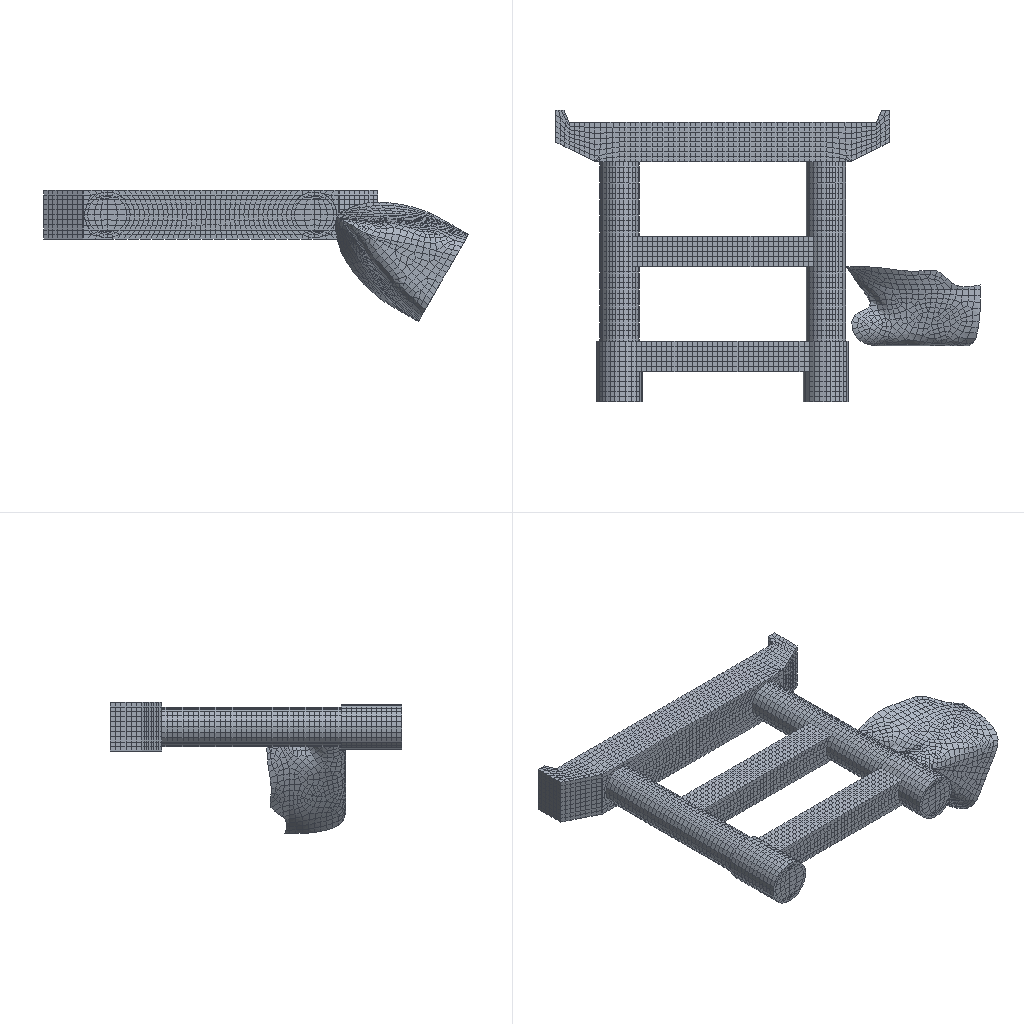Simulation study | abaqus
Set-up summary:
category,name,step,type,value,unit,region
solver,abaqus
solver,version,,,Abaqus/Explicit 2024
units,not stated in the deck,,not stated
analysis,deck,,transient,transient
load_step,Step-1,Step-1,transient,nlgeom=True
contact,interactions,,,general=1 pairs=0 ties=0
load_step,requested,,,1
mesh,nodes,,,29370
mesh,elements,,,26908
element_type,S3,,shell,56
element_type,S4R,,shell,1150
element_type,T3D2,,truss,11894
element_type,C3D8R,,solid,13808
load,load commands in deck,,count,1
bc,support commands in deck,,count,2
material,C40,,in results
material,HRE335,,in results
material,SHIP,,in results
check,setup vs results,,match,"per instance, exact: element labels, types and connectivity; labels of the nodes the elements use; coordinates of those nodes at SINGLE_PRECISION in 1 of 3 instance(s)"
Abaqus input file, long lists of numbers shortened:
*Heading
** Job name: Job-2 Model name: Model-1-Copy
** Generated by: Abaqus/CAE 2024
*Preprint, echo=NO, model=NO, history=NO, contact=NO
**
** PARTS
**
*Part, name=Bow
*Node
      1,   37800.219,        9242.,           0.
      2,       37800.,        9242.,           0.
** (1225 more lines like these left out)
*Element, type=S3
1,  47,  46,   4
2,  44,  49, 273
** (54 more lines like these left out)
*Element, type=S4R
  5,  19,  20, 352, 358
  6, 349,  64,  65, 358
** (1148 more lines like these left out)
*Nset, nset=BOW
 4,
*Nset, nset=Set-2, generate
    1,  1227,     1
*Elset, elset=Set-2, generate
    1,  1206,     1
*Nset, nset=Set-3, generate
    1,  1227,     1
** Section: Section-3
*Shell Section, elset=Set-2, material=Ship
50., 5
*End Part
**
*Part, name=Concrete
*Node
      1,       27500.,       -1500.,      -32750.
      2,       27500.,       -4000.,      -32750.
** (17351 more lines like these left out)
*Element, type=C3D8R
  1,     1,   285,  3364,   298,   329,  3544, 11654,  3384
  2,   285,   286,  3365,  3364,  3544,  3545, 11655, 11654
** (13806 more lines like these left out)
*Nset, nset=Set-1, generate
     1,  17353,      1
*Elset, elset=Set-1, generate
     1,  13808,      1
** Section: C40
*Solid Section, elset=Set-1, material=C40
,
*End Part
**
*Part, name=ganfjinlong
*Node
      1,      127050.,      -37500.,        4000.
      2,      130050.,      -37500.,        4000.
** (10788 more lines like these left out)
*Element, type=T3D2
1,    1, 1237
2, 1237, 1238
** (11892 more lines like these left out)
*Nset, nset=Set-1, generate
     1,  10790,      1
*Elset, elset=Set-1, generate
     1,  11894,      1
*Nset, nset=Set-2
   793,   794,   795,   796,   797,   798,   799,   800,   801,   802,   803,   804,   805,   806,   807,   808
   809,   810,   811,   812,   813,   814,   815,   816,   817,   818,   819,   820,   821,   822,   823,   824
** (225 more lines like these left out)
*Elset, elset=Set-2, generate
  7869,  11894,      1
** Section: HRB335
*Solid Section, elset=Set-1, material=HRE335
50.35,
*End Part
**
**
** ASSEMBLY
**
*Assembly, name=Assembly
**
*Instance, name=Concrete-1, part=Concrete
     116550.,           0.,           0.
     116550.,           0.,           0., 116549.,           0.,           0., 90.
*End Instance
**
*Instance, name=ganfjinlong-1, part=ganfjinlong
*End Instance
**
*Instance, name=Bow-1, part=Bow
215030.036,      -33500., -25289.
215030.036,      -33500., -25289., 215030.036, -33499., -25289., 210.
*End Instance
**
*Node
      1,   182294.281,      -24258.,       -6389.
*Nset, nset=Set-6, instance=Concrete-1
   235,   237,   238,   240,   241,   242,   243,   244,   245,   246,   247,   248,   249,   250,   251,   252
   253,   254,   255,   257,   260,   261,   262,   263,   265,   267,   268,   269,   270,   271,   273,   274
** (10 more lines like these left out)
*Elset, elset=Set-6, instance=Concrete-1
 10779, 10791, 10803, 10815, 10827, 10839, 10851, 10863, 10875, 10887, 10899, 10911, 10923, 10935, 10947, 10959
 10971, 10983, 11006, 11018, 11030, 11031, 11043, 11055, 11067, 11079, 11091, 11103, 11115, 11127, 11172, 11173
** (9 more lines like these left out)
*Nset, nset=Set-7, instance=Concrete-1
   37,   39,   40,   46,   54,   55,   56,   71,   74,   75,   78,   79,   81,   83,   85,   99
  100,  137,  141,  145,  169,  170,  172,  828,  829,  832,  866,  867, 1014, 1015, 1016, 1278
** (8 more lines like these left out)
*Elset, elset=Set-7, instance=Concrete-1
 4435, 4442, 4449, 4456, 4463, 4470, 4477, 4484, 4491, 4498, 4505, 4512, 4519, 4526, 4533, 4540
 4547, 4554, 4561, 4568, 4575, 4582, 4589, 4596, 4603, 4610, 4617, 4624, 4631, 4638, 4645, 4652
** (7 more lines like these left out)
*Nset, nset=Set-11, instance=Bow-1, generate
    1,  1227,     1
*Elset, elset=Set-11, instance=Bow-1, generate
    1,  1206,     1
*Nset, nset=m_Set-3, instance=ganfjinlong-1, generate
     1,  10790,      1
*Elset, elset=m_Set-3, instance=ganfjinlong-1, generate
     1,  11894,      1
*Nset, nset=m_Set-10, instance=ganfjinlong-1, generate
     1,  10790,      1
*Elset, elset=m_Set-10, instance=ganfjinlong-1, generate
     1,  11894,      1
*Nset, nset=s_Set-3, instance=Concrete-1, generate
     1,  17353,      1
*Elset, elset=s_Set-3, instance=Concrete-1, generate
     1,  13808,      1
*Nset, nset=s_Set-10, instance=Concrete-1, generate
     1,  17353,      1
*Elset, elset=s_Set-10, instance=Concrete-1, generate
     1,  13808,      1
*Nset, nset=_PickedSet378, internal
 1,
*Nset, nset=_PickedSet379, internal, instance=Bow-1, generate
    1,  1227,     1
*Elset, elset=_PickedSet379, internal, instance=Bow-1, generate
    1,  1206,     1
*Nset, nset=_PickedSet380, internal
 1,
*Elset, elset=_m_Surf-1_SNEG, internal, instance=Bow-1, generate
    1,  1206,     1
*Surface, type=ELEMENT, name=m_Surf-1
_m_Surf-1_SNEG, SNEG
*Elset, elset=_m_Surf-3_SNEG, internal, instance=Bow-1, generate
    1,  1206,     1
*Surface, type=ELEMENT, name=m_Surf-3
_m_Surf-3_SNEG, SNEG
*Elset, elset=_s_Surf-1_S3, internal, instance=Concrete-1
  7175,  7176,  7177,  7184,  7185,  7186,  7193,  7194,  7195,  7202,  7203,  7204,  7211,  7212,  7213,  7220
  7221,  7222,  7229,  7230,  7231,  7238,  7239,  7240,  7247,  7248,  7249,  7256,  7257,  7258,  7265,  7266
** (4 more lines like these left out)
*Elset, elset=_s_Surf-1_S6, internal, instance=Concrete-1
 7301, 7304, 7307, 7310, 7313, 7316, 7319, 7322, 7325, 7328, 7331, 7334, 7337, 7340, 7343, 7346
 7349, 7352, 7355, 7358, 7361, 7364, 7367, 7370, 7373, 7376, 7379, 7382, 7385, 7388, 7391, 7394
** (6 more lines like these left out)
*Surface, type=ELEMENT, name=s_Surf-1
_s_Surf-1_S3, S3
_s_Surf-1_S6, S6
*Elset, elset=_s_Surf-3_S6, internal, instance=Concrete-1
     1,     4,     7,    10,    13,    16,    19,    22,    25,    28,    31,    34,    37,    40,    43,    46
    49,    52,    55,    58,    61,    64,    67,    70,    73,    76,    79,    82,    85,    88,    91,    94
** (88 more lines like these left out)
*Elset, elset=_s_Surf-3_S5, internal, instance=Concrete-1
    16,    17,    18,    34,    35,    36,    52,    53,    54,    70,    71,    72,    88,    89,    90,   106
   107,   108,   124,   125,   126,   142,   143,   144,   160,   161,   162,   178,   179,   180,   196,   197
** (49 more lines like these left out)
*Elset, elset=_s_Surf-3_S1, internal, instance=Concrete-1
   868,   869,   870,   871,   872,   873,   874,   875,   876,   877,   878,   879,   880,   881,   882,   883
   884,   885,   886,   887,   888,   889,   890,   891,   892,   893,   894,   895,   896,   897,   898,   899
** (26 more lines like these left out)
*Elset, elset=_s_Surf-3_S3, internal, instance=Concrete-1
     1,     2,     3,    19,    20,    21,    37,    38,    39,    55,    56,    57,    73,    74,    75,    91
    92,    93,   109,   110,   111,   127,   128,   129,   145,   146,   147,   163,   164,   165,   181,   182
** (83 more lines like these left out)
*Elset, elset=_s_Surf-3_S2, internal, instance=Concrete-1
   613,   614,   615,   616,   617,   618,   619,   620,   621,   622,   623,   624,   625,   626,   627,   628
   629,   630,   631,   632,   633,   634,   635,   636,   637,   638,   639,   640,   641,   642,   643,   644
** (41 more lines like these left out)
*Elset, elset=_s_Surf-3_S4, internal, instance=Concrete-1
   924,   930,   936,   942,   948,   954,   960,   966,   972,   978,   984,   990,   996,  1002,  1008,  1014
  1020,  1026,  1032,  1038,  1044,  1050,  1056,  1062,  1068,  1074,  1080,  1086,  1092,  1098,  1104,  1110
** (121 more lines like these left out)
*Surface, type=ELEMENT, name=s_Surf-3
_s_Surf-3_S6, S6
_s_Surf-3_S5, S5
_s_Surf-3_S2, S2
_s_Surf-3_S4, S4
_s_Surf-3_S1, S1
_s_Surf-3_S3, S3
** Constraint: Constraint-2
*Embedded Element, host elset=s_Set-10
m_Set-10
** Constraint: Constraint-3
*Rigid Body, ref node=_PickedSet378, elset=_PickedSet379
*End Assembly
**
** MATERIALS
**
*Material, name=C40
*Density
 2.45e-09,
*Elastic
23500., 0.2
*Concrete Damaged Plasticity
30.,    0.1,   1.16, 0.6667, 0.0005
*Concrete Compression Hardening
 23.449,          0.
 25.046, 0.0003444
   26.06, 0.0004723
 26.595, 0.0006149
  26.752, 0.000769
 26.471, 0.0009366
 25.75,  0.001118
 24.752,  0.001307
 23.604,  0.001501
 22.396,  0.001697
 21.189,  0.001893
 20.019,  0.002088
 18.907,  0.002281
 17.865,  0.002472
 16.895,  0.002661
 15.996,  0.002848
 15.167,  0.003032
 14.403,  0.003214
  13.698,  0.003395
 13.048,  0.003574
 12.449,  0.003751
 11.895,  0.003927
 11.382,  0.004102
 10.908,  0.004275
*Concrete Tension Stiffening
  1.711,          0.
    1.966, 1.28235e-05
  2.185, 1.65417e-05
  2.345, 2.21036e-05
  2.408, 3.06091e-05
  2.331, 4.34029e-05
  2.194, 5.80792e-05
  2.041, 7.32033e-05
  1.893, 8.81996e-05
  1.756,  0.0001028
  1.633,  0.0001171
  1.524, 0.0001309
  1.427, 0.0001443
  1.341,  0.0001574
  1.264, 0.0001702
  1.196, 0.0001827
  1.135, 0.000195
  1.08, 0.0002071
  1.031, 0.0002191
 0.9862, 0.0002309
 0.9454, 0.0002426
 0.9082, 0.0002542
  0.8741,  0.0002657
 0.8427,  0.0002771
*Concrete Compression Damage
       0.,          0.
 0.1691, 0.0003444
 0.2072, 0.0004723
 0.2449, 0.0006149
 0.2815, 0.000769
 0.3185, 0.0009366
 0.3565,  0.001118
 0.3938,  0.001307
 0.4296,  0.001501
 0.4632,  0.001697
 0.4945,  0.001893
 0.5233,  0.002088
 0.5498,  0.002281
 0.574,  0.002472
 0.5963,  0.002661
 0.6166,  0.002848
 0.6353,  0.003032
 0.6524,  0.003214
  0.6681,  0.003395
 0.6826,  0.003574
 0.696,  0.003751
  0.7084,  0.003927
  0.7199,  0.004102
 0.7306,  0.004275
 0.7405,   0.004448
 0.7498,  0.004619
 0.7585,  0.00479
 0.7666,  0.00496
  0.7742,  0.005129
 0.7813,  0.005298
 0.788,   0.005465
 0.7944,  0.005633
 0.8003,  0.0058
 0.806,  0.005966
 0.8113,  0.006132
 0.8523,  0.007775
 0.8789,  0.009398
 0.8974,   0.01101
 0.911,   0.01262
 0.9215,   0.01422
** (20 more lines like these left out)
*Concrete Tension Damage
       0.,          0.
 0.0919, 1.28235e-05
 0.1044, 1.65417e-05
 0.1254, 2.21036e-05
  0.1592, 3.06091e-05
 0.2111, 4.34029e-05
 0.2674, 5.80792e-05
 0.321, 7.32033e-05
 0.3699, 8.81996e-05
 0.4137,  0.0001028
 0.4526,  0.0001171
 0.487, 0.0001309
  0.5176, 0.0001443
 0.5448,  0.0001574
 0.5692, 0.0001702
 0.591, 0.0001827
 0.6108, 0.000195
 0.6286, 0.0002071
 0.6448, 0.0002191
 0.6597, 0.0002309
 0.6732, 0.0002426
 0.6857, 0.0002542
  0.6973,  0.0002657
 0.7079,  0.0002771
 0.7178, 0.0002885
 0.727, 0.0002997
  0.7356, 0.0003109
 0.7436, 0.0003221
 0.7511, 0.0003332
 0.7582, 0.0003443
 0.7648, 0.0003553
 0.7711, 0.0003663
 0.777, 0.0003772
 0.7826, 0.0003882
 0.7879, 0.0003991
 0.8287, 0.000507
 0.8556, 0.0006138
 0.8747, 0.0007198
 0.8891, 0.0008255
 0.9002, 0.0009309
** (20 more lines like these left out)
*Material, name=HRE335
*Damage Initiation, criterion=DUCTILE
 0.1, 0.3333,    0.2
*Density
 7.85e-09,
*Elastic
200000., 0.28
*Plastic
335.,   0.
455., 0.06
*Material, name=Ship
*Density
 7.85e-09,
*Elastic
206000., 0.28
*Plastic
315.,0.
**
** INTERACTION PROPERTIES
**
*Surface Interaction, name=IntProp-1
*Friction
 0.2,
*Surface Behavior, pressure-overclosure=HARD
**
** BOUNDARY CONDITIONS
**
** Name: BC-1 Type: Symmetry/Antisymmetry/Encastre
*Boundary
Set-6, ENCASTRE
** Name: BC-2 Type: Symmetry/Antisymmetry/Encastre
*Boundary
Set-7, ENCASTRE
**
** PREDEFINED FIELDS
**
** Name: Predefined Field-1   Type: Velocity
*Initial Conditions, type=VELOCITY
_PickedSet380, 1, -5000.
** ----------------------------------------------------------------
**
** STEP: Step-1
**
*Step, name=Step-1, nlgeom=YES
*Dynamic, Explicit
, 0.01
*Bulk Viscosity
0.06, 1.2
** Mass Scaling: Semi-Automatic
**               Whole Model
*Fixed Mass Scaling, factor=10000.
**
** INTERACTIONS
**
** Interaction: Int-1
*Contact, op=NEW
*Contact Inclusions, ALL EXTERIOR
*Contact Property Assignment
 ,  , IntProp-1
**
** OUTPUT REQUESTS
**
*Restart, write, number interval=1, time marks=NO
**
** FIELD OUTPUT: F-Output-1
**
*Output, field
*Node Output, variable=PRESELECT
*Element Output, directions=YES, variable=PRESELECT
*Element Output, rebar, directions=YES, variable=PRESELECT
**
** HISTORY OUTPUT: H-Output-1
**
*Output, history, variable=PRESELECT
*End Step
Results summary:
result,step,Step-1,completed,increments=17 time=0.01/0.01
result,analysis,,,transient
result,last_loadstep,,,1
result,analysis steps,,count,1
result,primary field,,,"U, UR"
result,reaction total,,FX,0.0,model units
result,reaction total,,FY,0.0,model units
result,reaction total,,FZ,0.0,model units